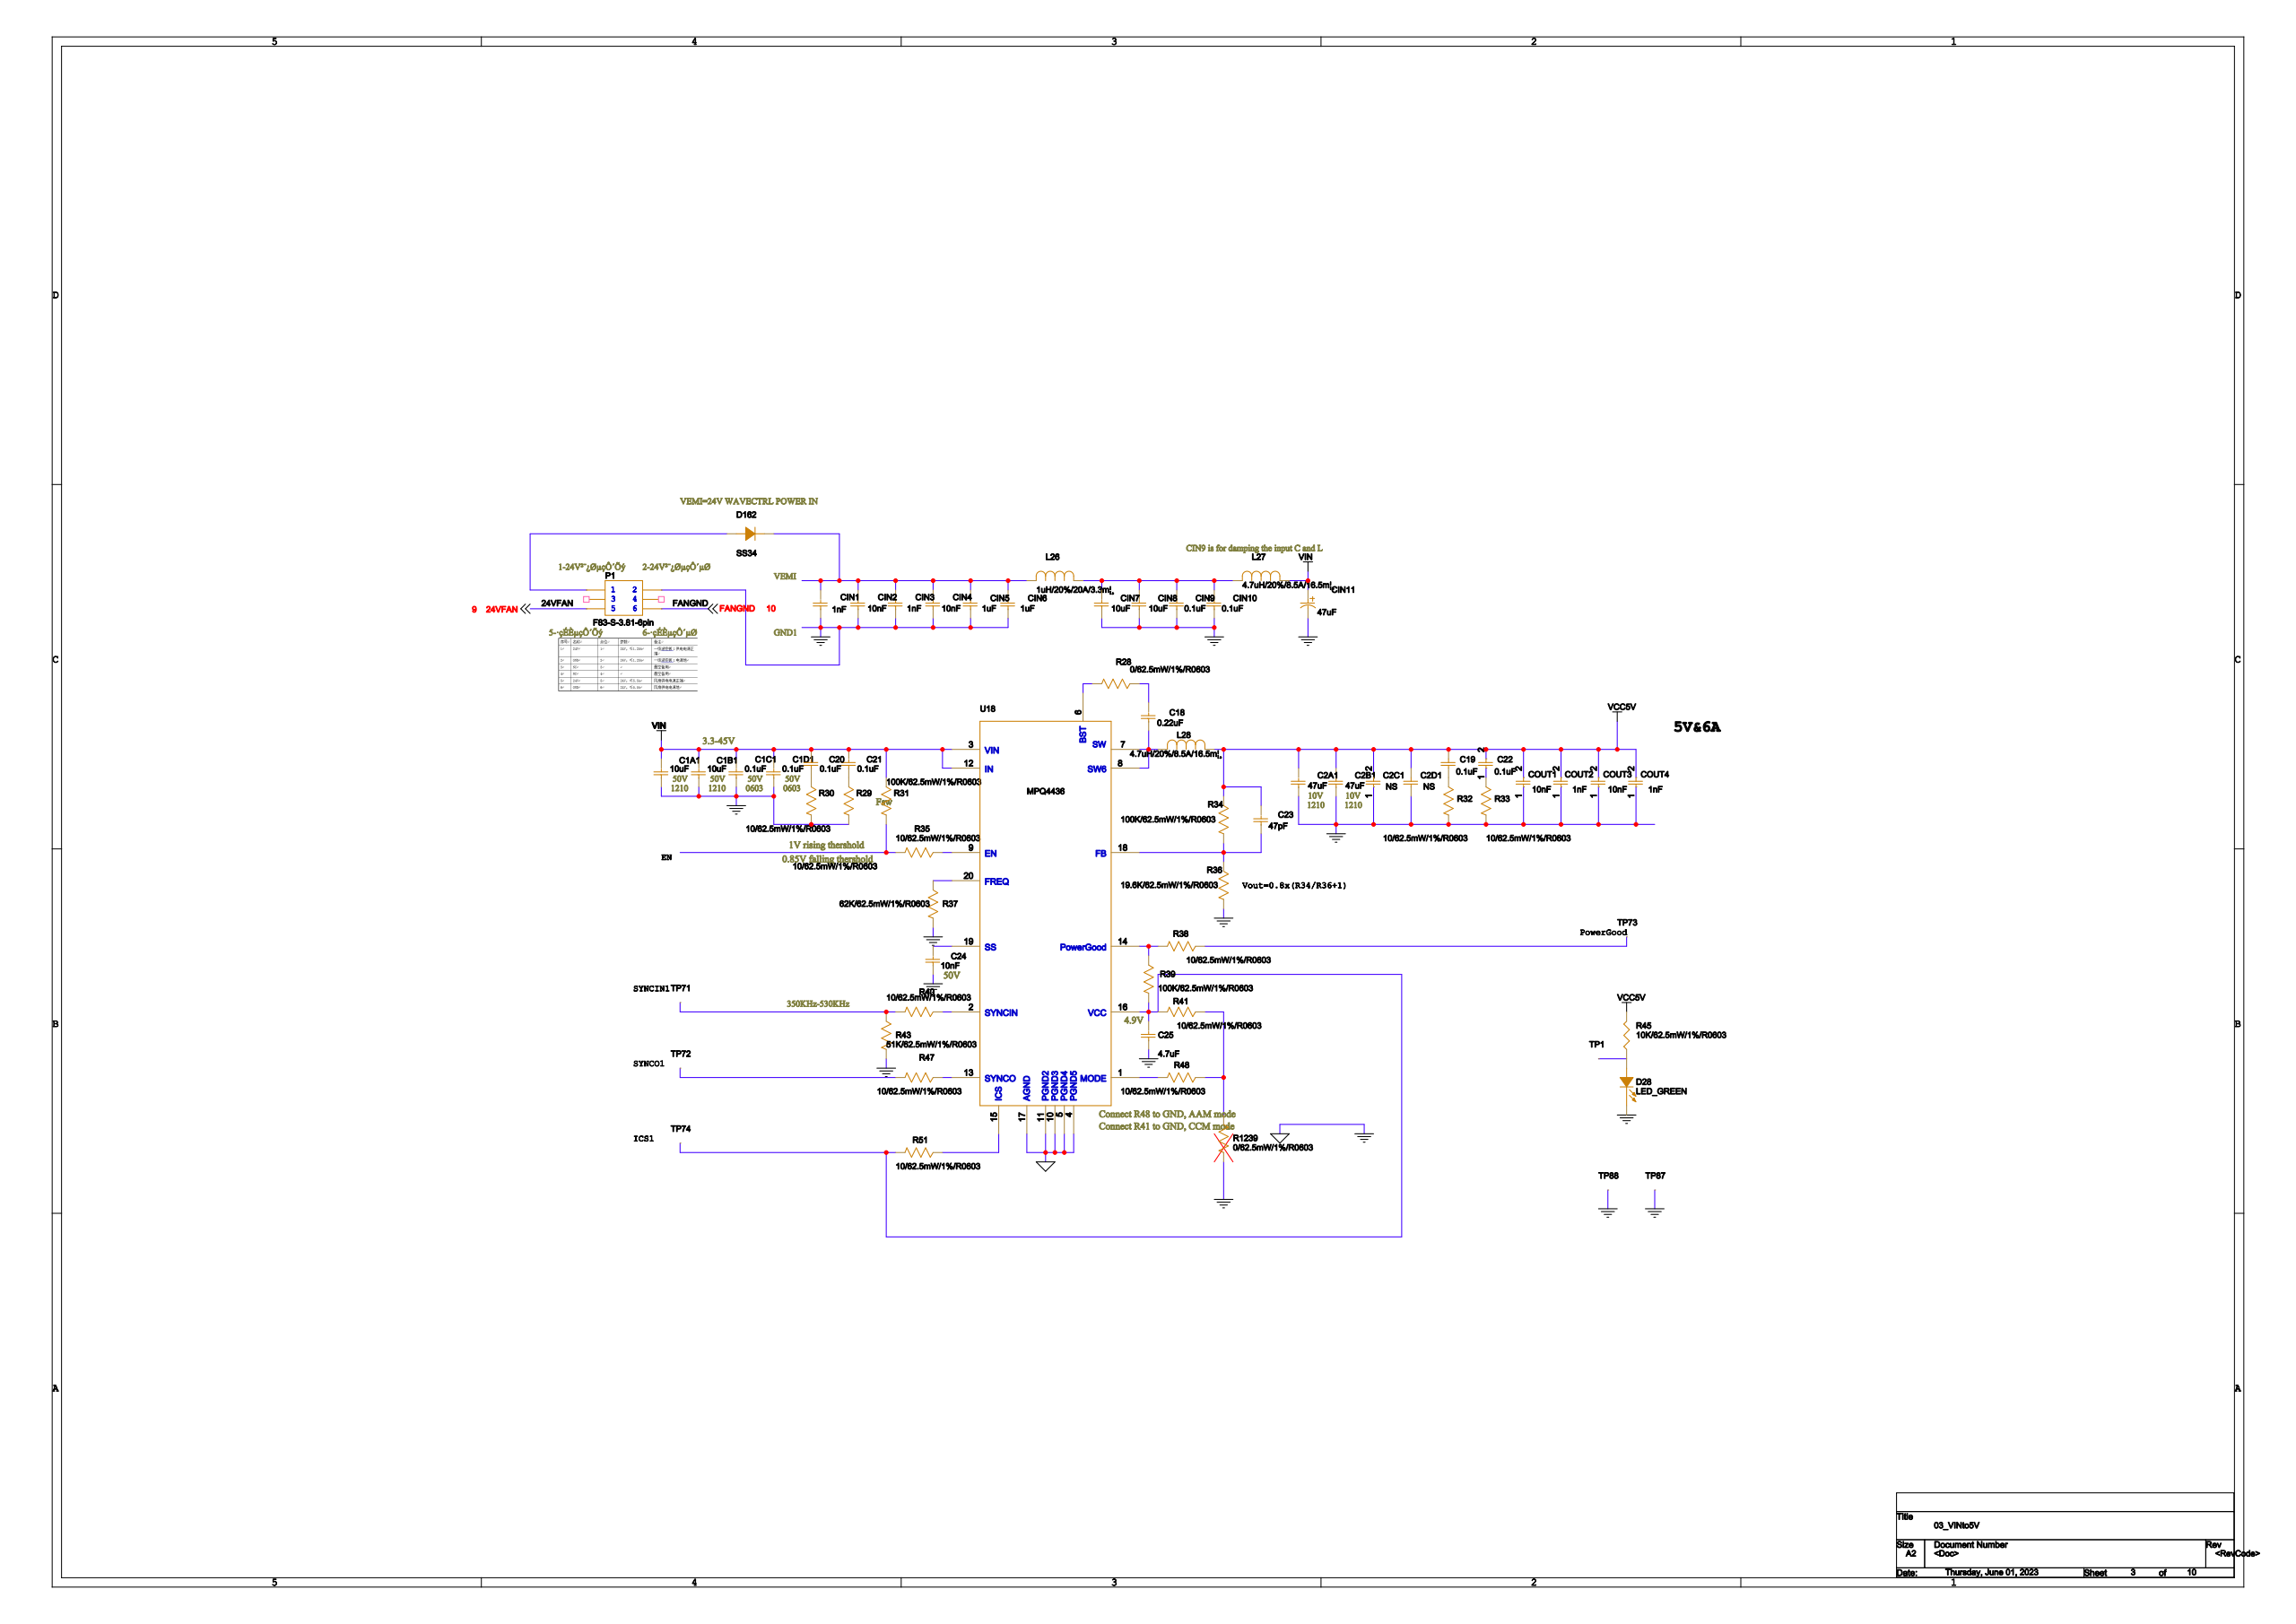Circuit board | Cadence Allegro | 480 parts | 625 nets | one sheet of the schematic
Parts on this sheet (reference | value | footprint):
C1A1 | CAP/1210 | 1210
C1B1 | CAP/1210 | 1210
C1C1 | CAP/0603 | 0603C
C1D1 | CAP/0603 | 0603C
C2A1 | CAP/1210 | 1210
C2B1 | CAP/1210 | 1210
C2C1 | CAP/0603 | 0603C
C2D1 | CAP/0603 | 0603C
C18 | CAP/0603 | 0603C
C19 | CAP/0603 | 0603C
C20 | CAP/0603 | 0603C
C21 | CAP/0603 | 0603C
C22 | CAP/0603 | 0603C
C23 | CAP/0603 | 0603C
C24 | CAP/0603 | 0603C
C25 | CAP/0603 | 0603C
CIN1 | CAP/0603 | 0603C
CIN2 | CAP/0603 | 0603C
CIN3 | CAP/0603 | 0603C
CIN4 | CAP/0603 | 0603C
CIN5 | CAP/0603 | 0805C
CIN6 | CAP/0603 | 0805C
CIN7 | CAP/0603 | 1206
CIN8 | CAP/0603 | 1206
CIN9 | CAP/0603 | 0603C
CIN10 | CAP/0603 | 0603C
CIN11 | CAP/ELECT/DIP/OD5.3P2.0 | AP-SMD_BD6_3-L6_6-W6_6-LS7_21
COUT1 | CAP/0603 | 0603C
COUT2 | CAP/0603 | 0603C
COUT3 | CAP/0603 | 0603C
COUT4 | CAP/0603 | 0603C
D28 | LED_GREEN | LED0805
D162 | SS34 | DO-214AC
L26 | CKST1004-1uH/M-B | SMD_10X11
L27 | CKST1004-4.7uH/M | SMD_10X11
L28 | CKST1004-4.7uH/M | SMD_10X11
P1 | F83-S-3.81-6pin | F83-S-3_81-6PIN
R28 | 0/62.5mW/1%/R0603 | 0603R
R29 | 10/62.5mW/1%/R0603 | 0603R
R30 | 10/62.5mW/1%/R0603 | 0603R
R31 | 100K/62.5mW/1%/R0603 | 0603R
R32 | 10/62.5mW/1%/R0603 | 0603R
R33 | 10/62.5mW/1%/R0603 | 0603R
R34 | 100K/62.5mW/1%/R0603 | 0603R
R35 | 10/62.5mW/1%/R0603 | 0603R
R36 | 19.6K/62.5mW/1%/R0603 | 0603R
R37 | 62K/62.5mW/1%/R0603 | 0603R
R38 | 10/62.5mW/1%/R0603 | 0603R
R39 | 100K/62.5mW/1%/R0603 | 0603R
R40 | 10/62.5mW/1%/R0603 | 0603R
R41 | 10/62.5mW/1%/R0603 | 0603R
R43 | 51K/62.5mW/1%/R0603 | 0603R
R45 | 10K/62.5mW/1%/R0603 | 0603R
R47 | 10/62.5mW/1%/R0603 | 0603R
R48 | 10/62.5mW/1%/R0603 | 0603R
R51 | 10/62.5mW/1%/R0603 | 0603R
R1239 | 0/62.5mW/1%/R0603 | 0603R
TP1 | TEST POINT A | TEST_12MM
TP71 | TEST POINT A | TEST_12MM
TP72 | TEST POINT A | TEST_12MM
TP73 | TEST POINT A | TEST_12MM
TP74 | TEST POINT A | TEST_12MM
TP87 | TEST POINT A | TEST_1MM
TP88 | TEST POINT A | TEST_1MM
U18 | MPQ4436 | QFN-4X4_MPQ4436-AEC1_MNP
Nets of these parts (net: part-pin ...):
AGND: C1A1-2 C1B1-2 C1C1-2 C1D1-2 C2A1-2 C2B1-2 C2C1-1 C2D1-1 C24-2 C25-2 CIN1-2 CIN2-2 CIN3-2 CIN4-2 CIN5-2 CIN6-2 CIN7-2 CIN8-2 CIN9-2 CIN10-2 CIN11-2 COUT1-1 COUT2-1 COUT3-1 COUT4-1 D28-2 P1-2 R29-2 R30-2 R32-2 R33-2 R36-1 R37-2 R43-1 R1239-2 TP87-1 TP88-1 U18-4 U18-5 U18-10 U18-11 U18-17
VCC5V: C2A1-1 C2B1-1 C2C1-2 C2D1-2 C19-2 C22-2 C23-1 COUT1-2 COUT2-2 COUT3-2 COUT4-2 L28-2 R34-2 R45-2
N23492270: D162-1 P1-1
N23491928: CIN1-1 CIN2-1 CIN3-1 CIN4-1 CIN5-1 CIN6-1 D162-2 L26-1
N23492006: R28-1 U18-6
N23491998: R35-2 U18-9
N23492020: C23-2 R34-1 R36-2 U18-18
N23491924: R37-1 U18-20
N23491980: R51-1 U18-15
VIN: C1A1-1 C1B1-1 C1C1-1 C1D1-1 C20-1 C21-1 CIN11-1 L27-2 R31-2 U18-3 U18-12
N23491986: R48-2 U18-1
N23491988: R38-2 R39-2 U18-14
N23491922: C24-1 U18-19
N23492014: C18-2 L28-1 U18-7 U18-8
N23491926: R40-2 U18-2
N23491976: R47-2 U18-13
N23491984: C25-1 R39-1 R41-2 R51-2 TP74-1 U18-16
N23492010: C18-1 R28-2
N234914480: C19-1 R32-1
N234914160: C20-2 R30-1
N234916911: C21-2 R29-1
N23492183: C22-1 R33-1
N23491954: CIN7-1 CIN8-1 CIN9-1 CIN10-1 L26-2 L27-1
N23491994: R41-1 R48-1 R1239-1
N23492000: R31-1 R35-1
N23492076: R38-1 TP73-1
N23491972: R40-1 R43-2 TP71-1
N23492221: D28-1 R45-1 TP1-1
N23491978: R47-1 TP72-1
FANGND: P1-6
24VFAN: P1-5